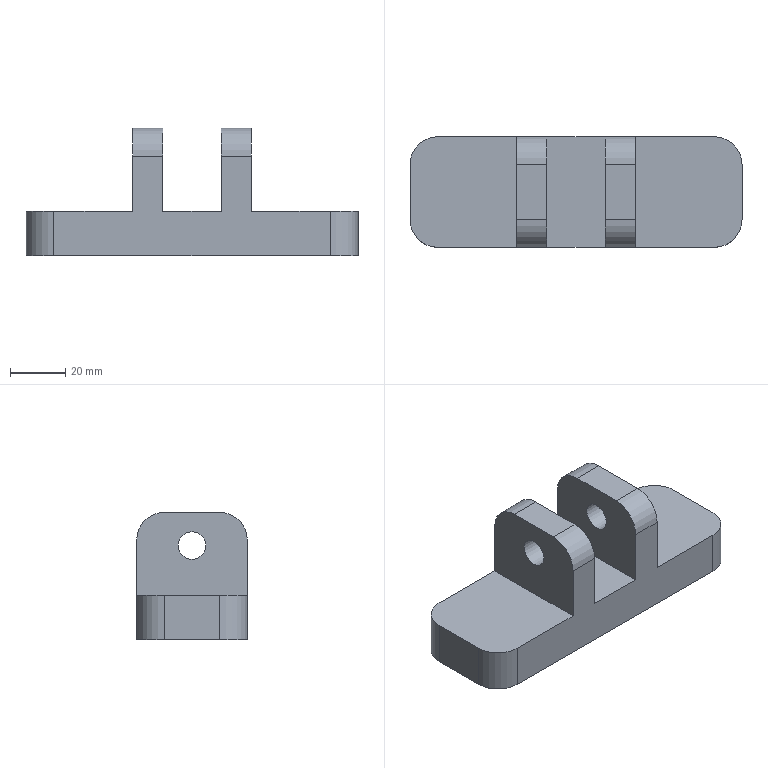NC program | NX | posted with a generic post | part box 120 x 40 x 46 mm
Lines 19 to 846 of 19901:
(ADAPTIVE_MILLING , TOOL : D16开粗)
N36 T02 M6
N38 G53
N40 G17 G0 G90 X-28.495 Y-40.02 S4500 M3
N42 G43 Z20. H2
N44 Z-26.
N46 G94 G1 X-28.48 Y-39.87 Z-26.937 F3000.
N48 X-28.464 Y-39.721 Z-27.308
N50 X-28.449 Y-39.572 Z-27.58
N52 X-28.434 Y-39.423 Z-27.8
N54 X-28.419 Y-39.274 Z-27.984
N56 X-28.404 Y-39.124 Z-28.142
N58 X-28.389 Y-38.975 Z-28.28
N60 X-28.374 Y-38.826 Z-28.4
N62 X-28.359 Y-38.677 Z-28.505
N64 X-28.343 Y-38.527 Z-28.598
N66 X-28.328 Y-38.378 Z-28.679
N68 X-28.313 Y-38.229 Z-28.75
N70 X-28.298 Y-38.08 Z-28.81
N72 X-28.283 Y-37.93 Z-28.862
N74 X-28.268 Y-37.781 Z-28.905
N76 X-28.253 Y-37.632 Z-28.939
N78 X-28.238 Y-37.483 Z-28.966
N80 X-28.222 Y-37.333 Z-28.985
N82 X-28.207 Y-37.184 Z-28.996
N84 X-28.192 Y-37.035 Z-29.
N86 X-27.96 Y-34.75
N88 G3 X-29.274 Y-32.998 R1.616
N90 X-33.053 Y-32.812 R30.645
N92 G1 X-39.412 Y-32.792
N94 X-61.887 Y-32.791
N96 G2 X-68.693 Y-29.137 R8.767
N98 X-70.931 Y-23.447 R12.623
N100 X-71.279 Y-17.763 R40.92
N102 G1 X-71.299 Y-11.163
N104 X-71.298 Y23.393
N106 G2 X-67.685 Y30.152 R8.778
N108 X-61.971 Y32.426 R12.581
N110 X-56.112 Y32.781 R41.464
N112 G1 X-49.137 Y32.799
N114 X61.886 Y32.791
N116 G2 X68.692 Y29.137 R8.766
N118 X70.935 Y23.424 R12.631
N120 X71.279 Y17.79 R40.982
N122 G1 X71.299 Y11.465
N124 X71.298 Y-23.378
N126 G2 X67.645 Y-30.185 R8.766
N128 X61.931 Y-32.427 R12.634
N130 X55.997 Y-32.774 R42.743
N132 G1 X49.122 Y-32.791
N134 X-27.311 Y-32.79
N136 G3 X-39.563 Y-32.593 R273.26
N138 G1 X-60.037 Y-32.592
N140 G2 X-68.805 Y-27.533 R10.212
N142 X-70.777 Y-21.44 R15.256
N144 X-71.086 Y-14.751 R58.815
N146 G1 X-71.099 Y-8.426
N148 X-71.098 Y21.668
N150 G2 X-66.042 Y30.3 R10.226
N152 X-60.025 Y32.266 R15.177
N154 X-53.637 Y32.583 R54.997
N156 G1 X-46.762 Y32.599
N158 X60.185 Y32.591
N160 G2 X68.829 Y27.494 R10.218
N162 X70.767 Y21.52 R15.204
N164 X71.084 Y15.032 R55.828
N166 G1 X71.099 Y9.232
N168 X71.098 Y-21.678
N170 G2 X65.962 Y-30.345 R10.223
N172 X59.978 Y-32.265 R15.287
N174 X53.064 Y-32.579 R60.014
N176 G1 X46.739 Y-32.591
N178 X-26.086 Y-32.59
N180 G3 X-40.413 Y-32.393 R535.751
N182 G1 X-58.462 Y-32.392
N184 G2 X-68.923 Y-26.041 R11.272
N186 X-70.614 Y-19.826 R17.76
N188 X-70.891 Y-12.185 R79.242
N190 G1 X-70.899 Y-6.41
N192 X-70.898 Y20.143
N194 G2 X-64.576 Y30.406 R11.261
N196 X-58.391 Y32.107 R17.661
N198 X-51.225 Y32.388 R73.205
N200 G1 X-45.45 Y32.398
N202 X58.662 Y32.391
N204 G2 X68.854 Y26.176 R11.237
N206 X70.583 Y20.102 R17.328
N208 X70.885 Y13.187 R66.446
N210 G1 X70.899 Y6.587
N212 X70.898 Y-20.153
N214 G2 X64.602 Y-30.388 R11.247
N216 X58.318 Y-32.108 R17.723
N218 X50.626 Y-32.383 R80.153
N220 G1 X44.851 Y-32.391
N222 X-25.035 Y-32.39
N224 X-34.168 Y-32.223
N226 X-41.888 Y-32.193
N228 X-56.987
N230 G2 X-62.563 Y-31.226 R13.756
N232 X-68.967 Y-24.705 R12.212
N234 X-70.438 Y-18.473 R20.206
N236 X-70.69 Y-10.704 R92.162
N238 G1 X-70.699 Y-4.929
N240 X-70.698 Y18.743
N242 G2 X-69.276 Y25.015 R12.961
N244 X-62.695 Y30.68 R12.482
N246 X-56.478 Y31.982 R21.635
N248 X-48.357 Y32.193 R112.946
N250 G1 X-43.407 Y32.198
N252 X57.286 Y32.19
N254 G2 X63.575 Y30.74 R12.89
N256 X69.21 Y24.117 R12.505
N258 X70.498 Y17.769 R22.064
N260 X70.694 Y9.623 R121.736
N262 G1 X70.699 Y4.948
N264 X70.697 Y-18.827
N266 G2 X69.125 Y-25.286 R12.764
N268 X62.56 Y-30.726 R12.562
N270 X56.258 Y-31.991 R22.207
N272 X47.487 Y-32.188 R130.953
N274 G1 X43.362 Y-32.191
N276 X-24.236 Y-32.189
N278 X-34.831 Y-32.02
N280 X-41.963 Y-31.994
N282 X-55.613 Y-31.993
N284 G2 X-60.638 Y-31.432 R17.397
N286 X-68.513 Y-24.534 R12.547
N288 X-70.19 Y-17.975 R20.237
N290 X-70.487 Y-10.059 R84.748
N292 G1 X-70.498 Y-4.559
N294 Y17.442
N296 G2 X-69.68 Y22.926 R15.632
N298 X-62.869 Y30.091 R12.636
N300 X-56.42 Y31.696 R20.514
N302 X-48.878 Y31.985 R82.683
N304 G1 X-42.003 Y31.998
N306 X56.036 Y31.99
N308 G2 X61.562 Y31.125 R15.334
N310 X68.612 Y24.321 R12.65
N312 X70.206 Y17.818 R20.687
N314 X70.488 Y9.951 R88.337
N316 G1 X70.498 Y4.451
N318 X70.497 Y-17.553
N320 G2 X69.614 Y-23.101 R15.249
N322 X62.847 Y-30.094 R12.653
N324 X56.396 Y-31.69 R20.582
N326 X48.429 Y-31.98 R87.328
N328 G1 X42.929 Y-31.99
N330 X-23.385 Y-31.989
N332 G2 X-33.923 Y-31.832 R874.419
N334 G3 X-49.088 Y-31.794 R944.969
N336 G2 X-56.587 Y-31.748 R216.51
N338 X-64.254 Y-29.071 R13.472
N340 X-68.978 Y-22.16 R14.117
N342 X-70.119 Y-15.5 R26.673
N344 X-70.296 Y-5.778 R173.557
N346 G1 X-70.298 Y-2.203
N348 X-70.297 Y16.268
N350 G2 X-69.697 Y21.54 R18.64
N352 X-62.521 Y29.745 R13.016
N354 X-55.893 Y31.458 R20.855
N356 X-47.553 Y31.786 R84.97
N358 G1 X-40.953 Y31.797
N360 X54.91 Y31.79
N362 G2 X60.249 Y31.129 R17.947
N364 X68.22 Y24.07 R13.009
N366 X69.97 Y17.275 R20.947
N368 X70.287 Y8.884 R88.25
N370 G1 X70.298 Y3.384
N372 X70.297 Y-16.427
N374 G2 X69.607 Y-21.836 R17.738
N376 X62.483 Y-29.755 R13.031
N378 X55.801 Y-31.46 R21.028
N380 X47.586 Y-31.778 R86.096
N382 G1 X40.986 Y-31.79
N384 X-22.485 Y-31.789
N386 G2 X-34.168 Y-31.632 R906.4
N388 G3 X-47.362 Y-31.594 R848.802
N390 G2 X-55.586 Y-31.554 R308.872
N392 X-62.467 Y-29.691 R14.738
N394 X-68.415 Y-22.518 R13.944
N396 X-69.85 Y-15.589 R24.559
N398 X-70.092 Y-6.319 R126.953
N400 G1 X-70.098 Y-1.094
N402 X-70.097 Y15.242
N404 G2 X-69.589 Y20.504 R21.438
N406 X-62.138 Y29.435 R13.405
N408 X-55.401 Y31.222 R21.242
N410 X-47.538 Y31.578 R77.171
N412 G1 X-39.838 Y31.597
N414 X53.786 Y31.59
N416 G2 X59.095 Y31.061 R21.109
N418 X67.964 Y23.574 R13.413
N420 X69.738 Y16.756 R21.472
N422 X70.082 Y8.567 R82.821
N424 G1 X70.097 Y2.242
N426 Y-15.178
N428 G2 X69.627 Y-20.344 R21.997
N430 X62.13 Y-29.432 R13.399
N432 X55.291 Y-31.227 R21.391
N434 X47.377 Y-31.571 R79.865
N436 G1 X39.677 Y-31.59
N438 X-21.885 Y-31.589
N440 G2 X-34.315 Y-31.433 R928.67
N442 G1 X-42.939 Y-31.394
N444 G2 X-54.537 Y-31.362 R722.301
N446 X-60.946 Y-29.987 R16.359
N448 X-67.913 Y-22.657 R14.012
N450 X-69.571 Y-15.678 R23.285
N452 X-69.885 Y-7.012 R97.267
N454 G1 X-69.898 Y-0.137
N456 X-69.897 Y14.168
N458 G2 X-69.496 Y19.368 R25.501
N460 X-61.56 Y29.235 R13.808
N462 X-54.64 Y31.023 R22.182
N464 X-46.351 Y31.379 R83.373
N466 G1 X-38.651 Y31.397
N468 X52.736 Y31.39
N470 G2 X58.008 Y30.96 R24.777
N472 X67.706 Y23.119 R13.793
N474 X69.529 Y16.082 R22.182
N476 X69.878 Y8.068 R82.45
N478 G1 X69.897 Y0.093
N480 X69.896 Y-14.302
N482 G2 X69.44 Y-19.621 R24.103
N484 X61.553 Y-29.231 R13.804
N486 X54.634 Y-31.015 R22.214
N488 X46.621 Y-31.369 R81.403
N490 G1 X38.646 Y-31.389
N492 X-21.46 Y-31.388
N494 G2 X-34.561 Y-31.233 R975.514
N496 G1 X-44.688 Y-31.194
N498 G2 X-54.062 Y-31.149 R356.626
N500 X-60.673 Y-29.658 R16.748
N502 X-67.681 Y-22.17 R14.377
N504 X-69.357 Y-15.093 R23.951
N506 X-69.685 Y-5.977 R101.058
N508 G1 X-69.697 Y0.898
N510 X-69.696 Y13.267
N512 G2 X-69.296 Y18.719 R27.895
N514 X-61.131 Y28.979 R14.164
N516 X-54.07 Y30.807 R22.749
N518 X-45.807 Y31.176 R82.954
N520 G1 X-37.557 Y31.196
N522 X51.886 Y31.189
N524 G2 X57.359 Y30.762 R26.877
N526 X67.486 Y22.611 R14.162
N528 X69.303 Y15.598 R22.718
N530 X69.677 Y7.21 R83.347
N532 G1 X69.697 Y-0.765
N534 X69.696 Y-13.328
N536 G2 X69.274 Y-18.826 R27.19
N538 X61.182 Y-28.947 R14.148
N540 X54.073 Y-30.798 R22.699
N542 X45.41 Y-31.171 R86.114
N544 G1 X37.71 Y-31.189
N546 X-20.86 Y-31.188
N548 G2 X-34.337 Y-31.037 R943.019
N550 G3 X-50.164 Y-30.993 R989.657
N552 G2 X-55.802 Y-30.727 R39.361
N554 X-67.329 Y-21.986 R14.563
N556 X-69.104 Y-14.908 R23.706
N558 X-69.476 Y-6.394 R86.921
N560 G1 X-69.497 Y1.856
N562 G2 X-69.461 Y14.617 R697.359
N564 X-68.257 Y20.971 R18.39
N566 X-60.49 Y28.83 R14.575
N568 X-53.338 Y30.613 R23.779
N570 X-45.049 Y30.974 R86.743
N572 G1 X-36.799 Y30.996
N574 X50.711 Y30.99
N576 G2 X56.293 Y30.647 R32.685
N578 X67.25 Y22.162 R14.512
N580 X69.097 Y14.976 R23.379
N582 X69.476 Y6.438 R85.803
N584 G1 X69.497 Y-1.812
N586 G2 X69.465 Y-14.502 R818.604
N588 X68.298 Y-20.864 R18.636
N590 X60.54 Y-28.799 R14.554
N592 X53.465 Y-30.59 R23.58
N594 X44.952 Y-30.968 R85.873
N596 G1 X36.702 Y-30.989
N598 X-20.31 Y-30.988
N600 G2 X-34.435 Y-30.837 R963.298
N602 G3 X-49.939 Y-30.792 R980.574
N604 G2 X-55.573 Y-30.467 R35.651
N606 X-67.03 Y-21.696 R14.843
N608 X-68.885 Y-14.431 R23.992
N610 X-69.272 Y-5.969 R85.324
N612 G1 X-69.297 Y2.556
N614 G2 X-69.254 Y14.067 R513.229
N616 X-68.012 Y20.565 R18.966
N618 X-60.044 Y28.601 R14.879
N620 X-52.719 Y30.409 R24.446
N622 X-44.255 Y30.774 R89.806
N624 G1 X-35.73 Y30.796
N626 X50.061 Y30.789
N628 G2 X55.792 Y30.429 R33.735
N630 X67.038 Y21.681 R14.833
N632 X68.887 Y14.415 R24.022
N634 X69.272 Y5.952 R85.818
N636 G1 X69.296 Y-1.748
N638 G2 X69.265 Y-13.752 R667.864
N640 X68.186 Y-20.107 R19.884
N642 X60.251 Y-28.5 R14.811
N644 X52.914 Y-30.379 R23.958
N646 X44.427 Y-30.765 R85.991
N648 G1 X35.902 Y-30.789
N650 X-19.785 Y-30.787
N652 G2 X-33.989 Y-30.643 R905.374
N654 G3 X-49.614 Y-30.59 R985.159
N656 G2 X-55.418 Y-30.194 R33.318
N658 X-66.77 Y-21.339 R15.111
N660 X-68.665 Y-13.981 R24.35
N662 X-69.071 Y-5.295 R85.885
N664 G1 X-69.096 Y3.505
N666 G2 X-69.044 Y13.617 R352.005
N668 X-67.764 Y20.185 R19.387
N670 X-59.807 Y28.288 R15.123
N672 X-52.473 Y30.167 R24.4
N674 X-44.037 Y30.568 R84.313
N676 G1 X-34.962 Y30.595
N678 X49.161 Y30.589
N680 G2 X54.996 Y30.264 R38.029
N682 X66.836 Y21.195 R15.154
N684 X68.678 Y13.875 R24.644
N686 X69.069 Y5.462 R85.964
N688 G1 X69.096 Y-3.613
N690 G2 X69.046 Y-13.552 R363.059
N692 X67.814 Y-20.054 R19.577
N694 X59.766 Y-28.298 R15.123
N696 X52.425 Y-30.164 R24.525
N698 X43.888 Y-30.562 R85.961
N700 G1 X35.088 Y-30.588
N702 X-18.635
N704 G2 X-33.764 Y-30.446 R900.131
N706 G3 X-48.89 Y-30.39 R948.428
N708 G2 X-54.771 Y-30.01 R35.78
N710 X-66.605 Y-20.787 R15.421
N712 X-68.461 Y-13.417 R25.102
N714 X-68.868 Y-4.78 R86.836
N716 X-68.858 Y12.567 R801.999
N718 X-67.796 Y19.08 R21.534
N720 X-59.434 Y28.042 R15.352
N722 X-51.957 Y29.958 R24.857
N724 X-43.02 Y30.37 R88.515
N726 G1 X-34.22 Y30.395
N728 X48.336 Y30.389
N730 G2 X54.347 Y30.076 R41.473
N732 X63.568 Y25.418 R15.54
N734 X67.623 Y17.917 R17.6
N736 X68.707 Y10.46 R35.639
N738 X68.893 Y-0.287 R214.956
N740 X68.857 Y-12.577 R641.025
N742 X67.824 Y-18.994 R21.581
N744 X59.547 Y-27.983 R15.327
N746 X52.053 Y-29.938 R24.629
N748 X42.967 Y-30.363 R87.854
N750 G1 X34.167 Y-30.388
N752 X-18.235
N754 G2 X-33.688 Y-30.248 R917.943
N756 G1 X-49.491 Y-30.176
N758 G2 X-55.787 Y-29.482 R26.997
N760 X-66.252 Y-20.666 R15.578
N762 X-68.213 Y-13.249 R24.835
N764 X-68.664 Y-4.415 R82.794
N766 X-68.66 Y11.842 R765.845
N768 X-67.688 Y18.322 R22.96
N770 X-59.089 Y27.79 R15.588
N772 X-51.641 Y29.727 R25.056
N774 X-42.806 Y30.165 R84.861
N776 G1 X-34.006 Y30.194
N778 X47.51 Y30.189
N780 G2 X53.649 Y29.897 R45.715
N782 X62.282 Y26.088 R16.108
N784 X67.156 Y18.32 R17.078
N786 X68.446 Y10.798 R32.424
N788 X68.691 Y-0.022 R171.414
N790 X68.653 Y-12.052 R545.91
N792 X67.579 Y-18.639 R22.117
N794 X59.135 Y-27.761 R15.584
N796 X51.764 Y-29.704 R24.869
N798 X43.13 Y-30.153 R81.304
N800 G1 X33.505 Y-30.188
N802 X-18.095
N804 G2 X-33.761 Y-30.048 R945.932
N806 G1 X-48.742 Y-29.977
N808 G2 X-55.071 Y-29.336 R29.098
N810 X-66.047 Y-20.23 R15.84
N812 X-68.002 Y-12.786 R25.323
N814 X-68.464 Y-3.702 R84.701
N816 X-68.451 Y11.472 R577.07
N818 X-67.424 Y18.044 R23.097
N820 X-58.699 Y27.565 R15.832
N822 X-51.198 Y29.513 R25.468
N824 X-42.389 Y29.961 R84.438
N826 G1 X-32.764 Y29.994
N828 X46.96 Y29.988
N830 G2 X53.272 Y29.674 R45.817
N832 X61.85 Y25.927 R16.41
N834 X66.874 Y18.098 R17.213
N836 X68.235 Y10.361 R32.489
N838 X68.489 Y-0.034 R162.063
N840 X68.451 Y-11.459 R486.743
N842 X67.41 Y-18.078 R23.037
N844 X58.737 Y-27.539 R15.821
N846 X51.291 Y-29.494 R25.325
N848 X42.557 Y-29.952 R82.326
N850 G1 X32.657 Y-29.987
N852 X-18.043
N854 G2 X-32.965 Y-29.857 R898.701
N856 G1 X-48.145 Y-29.777
N858 G2 X-54.551 Y-29.144 R30.331
N860 X-65.863 Y-19.76 R16.093
N862 X-67.806 Y-12.21 R26.014
N864 X-68.261 Y-3.276 R85.886
N866 X-68.249 Y10.899 R506.931
N868 X-67.235 Y17.549 R23.95
N870 X-58.396 Y27.305 R16.045
N872 X-50.832 Y29.292 R25.687
N874 X-42.023 Y29.757 R83.11
N876 G1 X-31.849 Y29.794
N878 X46.136 Y29.788
N880 G2 X52.574 Y29.497 R50.687
N882 X60.812 Y26.257 R17.025
N884 X66.426 Y18.362 R16.983
N886 X67.972 Y10.586 R30.435
N888 X68.283 Y0.569 R132.621
N890 X68.244 Y-11.031 R422.585
N892 X67.168 Y-17.745 R23.384
N894 X58.474 Y-27.261 R16.028
N896 X50.941 Y-29.27 R25.479
N898 X41.734 Y-29.753 R83.996
N900 G1 X31.834 Y-29.787
N902 X-17.991
N904 G2 X-32.716 Y-29.66 R899.522
N906 G1 X-47.624 Y-29.575
N908 G2 X-54.154 Y-28.926 R31.052
N910 X-65.595 Y-19.484 R16.301
N912 X-67.578 Y-11.914 R26.107
N914 X-68.059 Y-2.731 R85.348
N916 X-68.041 Y10.518 R408.196
N918 X-66.997 Y17.215 R24.208
N920 X-57.995 Y27.094 R16.271
N922 X-50.207 Y29.104 R26.342
N924 X-41.197 Y29.559 R87.741
N926 G1 X-31.297 Y29.594
N928 X45.336 Y29.588
N930 G2 X52. Y29.305 R54.728
N932 X60.118 Y26.285 R17.527
N934 X66.094 Y18.278 R17.018
N936 X67.713 Y10.695 R29.49
N938 X68.077 Y0.83 R115.354
N940 X68.033 Y-10.72 R339.442
N942 X66.891 Y-17.524 R23.369
N944 X58.039 Y-27.065 R16.262
N946 X50.303 Y-29.085 R26.19
N948 X41.194 Y-29.552 R86.807
N950 G1 X31.294 Y-29.587
N952 X-18.006
N954 G2 X-33.385 Y-29.454 R963.41
N956 G1 X-47.227 Y-29.372
N958 G2 X-53.83 Y-28.693 R31.203
N960 X-65.388 Y-19.083 R16.519
N962 X-67.371 Y-11.464 R26.56
N964 X-67.855 Y-2.381 R85.102
N966 X-67.838 Y10.018 R353.885
N968 X-66.784 Y16.814 R24.807
N970 X-57.721 Y26.829 R16.461
N972 X-49.963 Y28.872 R26.38
N974 X-40.581 Y29.359 R87.254
N976 G1 X-30.956 Y29.393
N978 X44.811 Y29.387
N980 G2 X51.624 Y29.088 R55.022
N982 X59.778 Y26.056 R17.799
N984 X65.873 Y17.905 R17.225
N986 X67.512 Y10.175 R30.024
N988 X67.878 Y0.01 R119.87
N990 X67.818 Y-10.464 R257.679
N992 X66.571 Y-17.426 R23.161
N994 X57.763 Y-26.802 R16.456
N996 X49.91 Y-28.87 R26.405
N998 X40.402 Y-29.353 R89.087
N1000 G1 X30.502 Y-29.387
N1002 X-17.948 Y-29.386
N1004 G2 X-32.364 Y-29.264 R913.591
N1006 G1 X-46.18 Y-29.18
N1008 G2 X-52.846 Y-28.609 R35.754
N1010 X-65.18 Y-18.693 R16.757
N1012 X-67.176 Y-10.923 R27.114
N1014 X-67.66 Y-1.415 R90.096
N1016 X-67.617 Y9.934 R259.101
N1018 X-66.442 Y16.81 R24.08
N1020 X-57.398 Y26.59 R16.657
N1022 X-49.696 Y28.643 R26.52
N1024 X-40.24 Y29.155 R85.431
N1026 X-29.79 Y29.193 R734.869
N1028 G1 X44.036 Y29.187
N1030 G2 X50.901 Y28.916 R60.739
N1032 X58.843 Y26.232 R18.531
N1034 X65.459 Y18.036 R17.146
N1036 X67.244 Y10.337 R28.778
N1038 X67.669 Y0.55 R103.168
N1040 X67.619 Y-9.899 R248.238
N1042 X66.41 Y-16.894 R24.002
N1044 X57.438 Y-26.564 R16.647
N1046 X49.564 Y-28.651 R26.648
N1048 X40.157 Y-29.149 R87.179
N1050 G1 X30.532 Y-29.186
N1052 X-17.943
N1054 G2 X-31.916 Y-29.069 R903.676
N1056 G1 X-45.459 Y-28.982
N1058 G2 X-52.154 Y-28.456 R38.65
N1060 X-61.791 Y-23.249 R17.085
N1062 X-66.028 Y-15.346 R19.333
N1064 X-67.251 Y-7.353 R38.336
N1066 X-67.489 Y4.692 R209.912
N1068 X-67.222 Y11.908 R64.582
N1070 X-64.612 Y19.849 R18.95
N1072 X-56.288 Y26.696 R17.279
N1074 X-48.303 Y28.548 R29.165
N1076 X-38.29 Y28.969 R107.484
N1078 G1 X-29.215 Y28.993
N1080 X43.51 Y28.987
N1082 G2 X50.451 Y28.711 R62.182
N1084 X58.341 Y26.111 R18.933
N1086 X65.194 Y17.787 R17.276
N1088 X67.026 Y9.999 R28.879
N1090 X67.465 Y0.288 R101.089
N1092 X67.401 Y-9.711 R198.424
N1094 X66.107 Y-16.765 R23.712
N1096 X57.075 Y-26.347 R16.843
N1098 X49.148 Y-28.442 R27.009
N1100 X39.967 Y-28.943 R85.954
N1102 X29.217 Y-28.986 R736.037
N1104 G1 X-17.958
N1106 G2 X-32.86 Y-28.86 R972.575
N1108 G1 X-44.663 Y-28.786
N1110 G2 X-51.414 Y-28.308 R42.501
N1112 X-60.461 Y-24.04 R17.629
N1114 X-65.527 Y-15.917 R18.617
N1116 X-66.969 Y-7.99 R34.47
N1118 X-67.283 Y3.153 R154.86
N1120 X-67.099 Y10.673 R86.711
N1122 X-65.099 Y18.243 R20.682
N1124 X-56.476 Y26.248 R17.17
N1126 X-48.657 Y28.252 R27.763
N1128 X-39.025 Y28.755 R90.485
N1130 G1 X-28.625 Y28.792
N1132 X42.71 Y28.787
N1134 G2 X49.778 Y28.533 R68.748
N1136 X57.673 Y26.089 R19.607
N1138 X64.895 Y17.629 R17.357
N1140 X66.797 Y9.778 R28.715
N1142 X67.261 Y0.018 R97.923
N1144 X67.186 Y-9.455 R165.994
N1146 X65.801 Y-16.643 R23.568
N1148 X56.758 Y-26.113 R17.028
N1150 X48.787 Y-28.228 R27.253
N1152 X39.43 Y-28.742 R86.53
N1154 X28.631 Y-28.786 R739.901
N1156 G1 X-17.944
N1158 X-34.027 Y-28.649
N1160 G2 X-46.065 Y-28.547 R895.515
N1162 X-52.993 Y-27.666 R29.894
N1164 X-64.396 Y-17.92 R17.227
N1166 X-66.534 Y-9.827 R27.66
N1168 X-67.047 Y-0.546 R87.013
N1170 X-66.972 Y9.177 R151.109
N1172 X-65.551 Y16.385 R23.654
N1174 X-56.376 Y25.919 R17.217
N1176 X-48.452 Y28.019 R27.535
N1178 X-38.972 Y28.547 R86.592
N1180 X-27.947 Y28.592 R745.421
N1182 G1 X42.16 Y28.586
N1184 G2 X49.452 Y28.317 R68.879
N1186 X57.324 Y25.878 R19.841
N1188 X64.655 Y17.333 R17.516
N1190 X66.601 Y9.266 R29.131
N1192 X67.057 Y-0.195 R97.799
N1194 X66.963 Y-9.317 R137.485
N1196 X65.432 Y-16.676 R23.138
N1198 X56.345 Y-25.925 R17.229
N1200 X48.321 Y-28.027 R27.76
N1202 X38.714 Y-28.544 R89.393
N1204 X27.939 Y-28.585 R741.437
N1206 G1 X-17.961
N1208 X-30.16 Y-28.488
N1210 X-43.595 Y-28.388
N1212 G2 X-50.546 Y-27.906 R45.118
N1214 X-59.405 Y-23.972 R18.243
N1216 X-64.932 Y-15.692 R18.626
N1218 X-66.519 Y-7.616 R33.519
N1220 X-66.875 Y3.225 R135.719
N1222 X-66.604 Y10.641 R65.561
N1224 X-64.091 Y18.619 R19.963
N1226 X-55.533 Y25.921 R17.693
N1228 X-47.494 Y27.879 R29.254
N1230 X-37.685 Y28.357 R98.352
N1232 G1 X-27.31 Y28.391
N1234 X41.66 Y28.386
N1236 G2 X48.952 Y28.121 R71.042
N1238 X56.76 Y25.791 R20.34
N1240 X64.334 Y17.231 R17.594
N1242 X66.345 Y9.283 R28.593
N1244 X66.849 Y-0.199 R90.998
N1246 X66.733 Y-9.246 R116.358
N1248 X65.081 Y-16.653 R22.72
N1250 X56.09 Y-25.668 R17.395
N1252 X48.173 Y-27.788 R27.677
N1254 X38.544 Y-28.338 R85.927
N1256 X27.319 Y-28.385 R745.688
N1258 G1 X-17.956
N1260 X-29.02 Y-28.299
N1262 X-43.848 Y-28.177
N1264 G2 X-50.788 Y-27.584 R39.755
N1266 X-60.244 Y-22.699 R17.94
N1268 X-64.997 Y-14.488 R19.593
N1270 X-66.378 Y-6.422 R37.111
N1272 X-66.566 Y8.245 R140.445
N1274 X-65.161 Y15.583 R24.648
N1276 X-55.766 Y25.455 R17.54
N1278 X-47.823 Y27.583 R27.91
N1280 X-38.495 Y28.137 R83.81
N1282 X-21.749 Y28.193 R998.59
N1284 G1 X-8.352
N1286 X-4.761 Y28.19
N1288 X10.388
N1290 X23.774 Y28.191
N1292 X27.664 Y28.188
N1294 X40.863 Y28.186
N1296 G2 X48.43 Y27.928 R76.499
N1298 X56.303 Y25.644 R20.816
N1300 X64.098 Y16.939 R17.734
N1302 X66.149 Y8.796 R28.984
N1304 X66.652 Y-0.987 R94.595
N1306 X66.485 Y-9.357 R90.495
N1308 X64.555 Y-16.999 R21.868
N1310 X55.717 Y-25.468 R17.601
N1312 X47.671 Y-27.595 R28.175
N1314 X38.341 Y-28.132 R86.033
N1316 X21.831 Y-28.186 R982.053
N1318 G1 X7.477 Y-28.188
N1320 X3.887 Y-28.186
N1322 X-10.337
N1324 G2 X-31.139 Y-28.078 R965.223
N1326 G1 X-43.451 Y-27.976
N1328 G2 X-50.514 Y-27.357 R39.853
N1330 X-60.051 Y-22.372 R18.088
N1332 X-64.753 Y-14.238 R19.762
N1334 X-66.179 Y-5.927 R37.473
N1336 X-66.35 Y7.99 R126.357
N1338 X-64.889 Y15.391 R24.58
N1340 X-55.458 Y25.227 R17.698
N1342 X-47.27 Y27.397 R28.395
N1344 X-37.615 Y27.942 R88.59
N1346 X-23.314 Y27.998 R947.443
N1348 G1 X-23.117 Y28.028
N1350 G3 X-22.265 Y28.588 R1.604
N1352 G1 X-21.411 Y29.676
N1354 X-19.439 Y32.187 Z-28.9
N1356 X-19.257 Y32.419 F15000.
N1358 X-19.066 Y32.644
N1360 G2 X-18.037 Y33.108 R1.603
N1362 G1 X-15.386 Y33.278
N1364 G2 X-13.959 Y32.576 R1.601
N1366 G1 X-13.702 Y32.196
N1368 X-11.914 Y29.55 Z-29. F3000.
N1370 X-11.645 Y29.149
N1372 X-11.365 Y28.754
N1374 G3 X-10.306 Y28.198 R1.602
N1376 X-5.191 Y28.001 R48.101
N1378 G1 X-0.737 Y27.99
N1380 X8.738 Y28.003
N1382 X8.861 Y28.023
N1384 G3 X9.605 Y31.087 R1.76
N1386 X8.335 Y31.5 Z-28.957 R1.854
N1388 G1 X6.51 Y31.514 Z-28.9
N1390 X-6.817 Y31.616 F15000.
N1392 X-9.394 Y31.636 Z-28.981 F3000.
N1394 G3 X-9.999 Y31.533 Z-29. R1.915
N1396 X-9.585 Y28.125 R1.76
N1398 X-3.985 Y27.81 R40.581
N1400 X7.953 Y27.814 R504.393
N1402 X9.047 Y28.07 R8.417
N1404 G1 X10.417 Y28.193
N1406 G3 X10.268 Y31.706 R1.76
N1408 G1 X7.075 Y31.676 Z-28.9
N1410 X-6.598 Y31.551 F15000.
N1412 X-7.656 Y31.544 Z-28.933 F3000.
N1414 X-8.713 Y31.526 Z-28.966
N1416 G3 X-9.702 Y31.145 Z-29. R1.761
N1418 X-9.045 Y28.07 R1.76
N1420 X-5.723 Y27.682 R15.275
N1422 X7.074 Y27.617 R328.219
N1424 X7.71 Y27.708 R3.624
N1426 X8.504 Y30.409 R1.72
N1428 X7.194 Y31.057 Z-28.953 R1.733
N1430 G1 X5.511 Y31.092 Z-28.9
N1432 X-6.035 Y31.331 F15000.
N1434 X-8.378 Y31.374 Z-28.973 F3000.
N1436 G3 X-9.186 Y31.144 Z-29. R1.725
N1438 X-8.755 Y27.994 R1.72
N1440 X-5.352 Y27.518 R14.723
N1442 X6.503 Y27.432 R201.773
N1444 X7.455 Y27.591 R3.948
N1446 X8.222 Y30.173 R1.76
N1448 X6.795 Y30.964 Z-28.947 R1.771
N1450 G1 X5.299 Y31. Z-28.9
N1452 X-5.889 Y31.267 F15000.
N1454 X-6.849 Y31.292 Z-28.93 F3000.
N1456 X-7.809 Y31.308 Z-28.96
N1458 G3 X-8.959 Y30.833 Z-29. R1.76
N1460 X-8.198 Y27.848 R1.76
N1462 X-4.629 Y27.332 R15.348
N1464 X5.945 Y27.246 R142.08
N1466 X7.073 Y27.425 R4.753
N1468 G2 X8.208 Y27.851 R5.381
N1470 G3 X9.018 Y30.788 R1.76
N1472 X7.741 Y31.314 Z-28.956 R1.778
N1474 G1 X5.968 Y31.291 Z-28.9
N1476 X-5.601 Y31.142 F15000.
N1478 X-7.231 Y31.117 Z-28.951 F3000.
N1480 G3 X-8.551 Y30.382 Z-29. R1.759
N1482 X-7.819 Y27.749 R1.76
N1484 X-5.04 Y27.224 R10.254
N1486 X5.47 Y27.062 R102.51
N1488 X7.095 Y27.434 R3.768
N1490 X7.865 Y30.013 R1.76
N1492 X6.43 Y30.808 Z-28.947 R1.77
N1494 G1 X4.944 Y30.839 Z-28.9
N1496 X-5.41 Y31.059 F15000.
N1498 X-6.26 Y31.079 Z-28.927 F3000.
N1500 X-7.11 Y31.089 Z-28.953
N1502 G3 X-8.408 Y30.449 Z-29. R1.759
N1504 X-7.75 Y27.719 R1.76
N1506 X-5.088 Y27.102 R8.821
N1508 X2.679 Y26.813 R77.353
N1510 X6.12 Y27.023 R18.561
N1512 G1 X6.542 Y27.176
N1514 G3 X7.118 Y29.602 R1.67
N1516 X5.815 Y30.314 Z-28.952 R1.682
N1518 G1 X4.162 Y30.379 Z-28.9
N1520 X-4.704 Y30.728 F15000.
N1522 X-5.782 Y30.773 Z-28.934 F3000.
N1524 X-6.86 Y30.808 Z-28.968
N1526 G3 X-7.825 Y30.483 Z-29. R1.671
N1528 X-7.498 Y27.609 R1.67
N1530 X-4.639 Y26.927 R9.284
N1532 X4.762 Y26.71 R63.118
N1534 X6.376 Y27.066 R4.247
N1536 X7.016 Y29.397 R1.76
N1538 X5.538 Y30.329 Z-28.943 R1.77
N1540 G1 X4.175 Y30.387 Z-28.9
N1542 X-4.782 Y30.772 F15000.
N1544 X-6.497 Y30.841 Z-28.954 F3000.
N1546 G3 X-7.799 Y30.243 Z-29. R1.759
N1548 X-7.177 Y27.47 R1.76
N1550 X-4.289 Y26.759 R9.502
N1552 X4.442 Y26.538 R52.187
N1554 X6.134 Y26.913 R4.703
N1556 G1 X6.704 Y27.264
N1558 G3 X7.492 Y29.816 R1.76
N1560 X6.011 Y30.638 Z-28.945 R1.77
N1562 G1 X4.585 Y30.645 Z-28.9
N1564 X-4.633 Y30.687 F15000.
N1566 X-6.217 Y30.689 Z-28.95 F3000.
N1568 G3 X-7.576 Y29.939 Z-29. R1.759
N1570 X-6.833 Y27.32 R1.76
N1572 X-3.924 Y26.588 R9.619
N1574 X4.284 Y26.382 R42.683
N1576 X5.917 Y26.775 R4.431
N1578 G1 X6.171 Y26.935
N1580 G3 X6.768 Y29.275 R1.76
N1582 X5.278 Y30.181 Z-28.943 R1.77
N1584 G1 X3.91 Y30.22 Z-28.9
N1586 X-4.248 Y30.449 F15000.
N1588 X-5.763 Y30.486 Z-28.948 F3000.
N1590 G3 X-7.176 Y29.709 Z-29. R1.759
N1592 X-6.656 Y27.243 R1.76
N1594 X-4.24 Y26.515 R7.401
N1596 X4.071 Y26.223 R36.003
N1598 X5.657 Y26.61 R4.504
N1600 G1 X5.932 Y26.784
N1602 G3 X6.541 Y29.102 R1.76
N1604 X5.061 Y30.029 Z-28.943 R1.77
N1606 G1 X3.696 Y30.084 Z-28.9
N1608 X-4.176 Y30.404 F15000.
N1610 X-5.698 Y30.46 Z-28.948 F3000.
N1612 G3 X-7.117 Y29.707 Z-29. R1.759
N1614 X-6.614 Y27.217 R1.76
N1616 X-4.36 Y26.428 R6.435
N1618 X3.965 Y26.078 R30.673
N1620 X5.485 Y26.493 R3.933
N1622 G1 X5.548 Y26.534
N1624 G3 X6.039 Y28.713 R1.76
N1626 X4.585 Y29.679 Z-28.943 R1.77
N1628 G1 X3.222 Y29.771 Z-28.9
N1630 X-3.943 Y30.254 F15000.
N1632 X-5.481 Y30.353 Z-28.948 F3000.
N1634 G3 X-6.909 Y29.653 Z-29. R1.759
N1636 X-6.445 Y27.109 R1.76
N1638 X-4.032 Y26.254 R6.813
N1640 X3.756 Y25.922 R27.382
N1642 X5.37 Y26.391 R4.014
N1644 G1 X5.452 Y26.449
N1646 G3 X5.876 Y28.635 R1.71
N1648 X4.503 Y29.496 Z-28.947 R1.72
N1650 G1 X3.002 Y29.595 Z-28.9
N1652 X-3.591 Y30.031 F15000.
N1654 X-4.457 Y30.09 Z-28.927 F3000.
N1656 X-5.324 Y30.14 Z-28.954
N1658 G3 X-6.616 Y29.571 Z-29. R1.709
N1660 X-6.255 Y26.989 R1.71
N1662 X-3.819 Y26.102 R6.924
N1664 X3.655 Y25.784 R24.245
N1666 X5.242 Y26.275 R4.012
N1668 G1 X5.323 Y26.335
N1670 G3 X5.767 Y28.496 R1.76
N1672 X4.325 Y29.447 Z-28.943 R1.77
N1674 G1 X2.941 Y29.544 Z-28.9
N1676 X-3.536 Y29.996 F15000.
N1678 X-5.076 Y30.098 Z-28.948 F3000.
N1680 G3 X-6.505 Y29.404 Z-29. R1.759
N1682 X-6.044 Y26.855 R1.76
N1684 X-3.6 Y25.946 R6.991